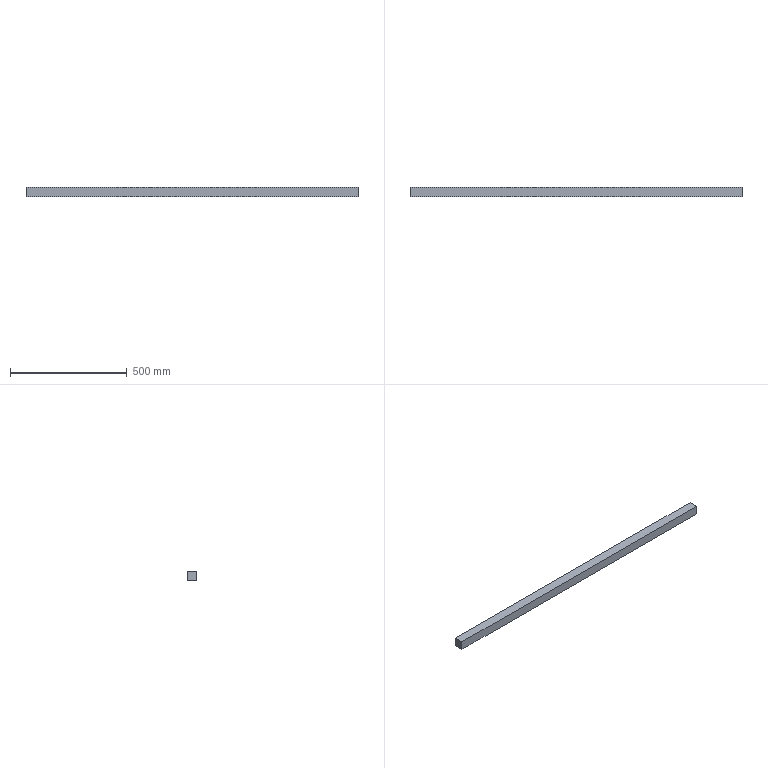Part | NX | features 凸台-拉伸2[1] 2 | 1 solid | 6 faces | box 1420 x 40 x 40 mm | volume 2272000 mm3 | plane 6
STEP:
#1=CARTESIAN_POINT('',(4293.,-600.,1387.015));
#2=VERTEX_POINT('',#1);
#3=CARTESIAN_POINT('',(4293.,-600.,1427.015));
#4=VERTEX_POINT('',#3);
#5=CARTESIAN_POINT('',(4293.,-600.,1427.015));
#6=DIRECTION('',(0.,0.,1.));
#7=VECTOR('',#6,1000.);
#8=LINE('',#5,#7);
#9=EDGE_CURVE('',#2,#4,#8,.T.);
#10=ORIENTED_EDGE('',*,*,#9,.F.);
#11=CARTESIAN_POINT('',(4293.,-560.,1387.015));
#12=VERTEX_POINT('',#11);
#13=CARTESIAN_POINT('',(4293.,-600.,1387.015));
#14=DIRECTION('',(0.,-1.,0.));
#15=VECTOR('',#14,1000.);
#16=LINE('',#13,#15);
#17=EDGE_CURVE('',#12,#2,#16,.T.);
#18=ORIENTED_EDGE('',*,*,#17,.F.);
#19=CARTESIAN_POINT('',(4293.,-560.,1427.015));
#20=VERTEX_POINT('',#19);
#21=CARTESIAN_POINT('',(4293.,-560.,1427.015));
#22=DIRECTION('',(0.,0.,-1.));
#23=VECTOR('',#22,1000.);
#24=LINE('',#21,#23);
#25=EDGE_CURVE('',#20,#12,#24,.T.);
#26=ORIENTED_EDGE('',*,*,#25,.F.);
#27=CARTESIAN_POINT('',(4293.,-600.,1427.015));
#28=DIRECTION('',(0.,1.,0.));
#29=VECTOR('',#28,1000.);
#30=LINE('',#27,#29);
#31=EDGE_CURVE('',#4,#20,#30,.T.);
#32=ORIENTED_EDGE('',*,*,#31,.F.);
#33=EDGE_LOOP('',(#10,#18,#26,#32));
#34=FACE_BOUND('',#33,.T.);
#35=CARTESIAN_POINT('',(4293.,-600.,1427.015));
#36=DIRECTION('',(-1.,0.,0.));
#37=DIRECTION('',(0.,0.,1.));
#38=AXIS2_PLACEMENT_3D('',#35,#36,#37);
#39=PLANE('',#38);
#40=ADVANCED_FACE('',(#34),#39,.F.);
#41=CARTESIAN_POINT('',(2873.,-600.,1427.015));
#42=VERTEX_POINT('',#41);
#43=CARTESIAN_POINT('',(4349.569,-600.,1427.015));
#44=DIRECTION('',(-1.,0.,0.));
#45=VECTOR('',#44,1000.);
#46=LINE('',#43,#45);
#47=EDGE_CURVE('',#4,#42,#46,.T.);
#48=ORIENTED_EDGE('',*,*,#47,.F.);
#49=ORIENTED_EDGE('',*,*,#31,.T.);
#50=CARTESIAN_POINT('',(2873.,-560.,1427.015));
#51=VERTEX_POINT('',#50);
#52=CARTESIAN_POINT('',(4349.569,-560.,1427.015));
#53=DIRECTION('',(-1.,0.,0.));
#54=VECTOR('',#53,1000.);
#55=LINE('',#52,#54);
#56=EDGE_CURVE('',#20,#51,#55,.T.);
#57=ORIENTED_EDGE('',*,*,#56,.T.);
#58=CARTESIAN_POINT('',(2873.,-600.,1427.015));
#59=DIRECTION('',(0.,-1.,0.));
#60=VECTOR('',#59,1000.);
#61=LINE('',#58,#60);
#62=EDGE_CURVE('',#51,#42,#61,.T.);
#63=ORIENTED_EDGE('',*,*,#62,.T.);
#64=EDGE_LOOP('',(#48,#49,#57,#63));
#65=FACE_BOUND('',#64,.T.);
#66=CARTESIAN_POINT('',(4349.569,-600.,1427.015));
#67=DIRECTION('',(0.,0.,-1.));
#68=DIRECTION('',(-1.,0.,0.));
#69=AXIS2_PLACEMENT_3D('',#66,#67,#68);
#70=PLANE('',#69);
#71=ADVANCED_FACE('',(#65),#70,.F.);
#72=CARTESIAN_POINT('',(2873.,-600.,1387.015));
#73=VERTEX_POINT('',#72);
#74=CARTESIAN_POINT('',(4349.569,-600.,1387.015));
#75=DIRECTION('',(-1.,0.,0.));
#76=VECTOR('',#75,1000.);
#77=LINE('',#74,#76);
#78=EDGE_CURVE('',#2,#73,#77,.T.);
#79=ORIENTED_EDGE('',*,*,#78,.F.);
#80=ORIENTED_EDGE('',*,*,#9,.T.);
#81=ORIENTED_EDGE('',*,*,#47,.T.);
#82=CARTESIAN_POINT('',(2873.,-600.,1427.015));
#83=DIRECTION('',(0.,0.,-1.));
#84=VECTOR('',#83,1000.);
#85=LINE('',#82,#84);
#86=EDGE_CURVE('',#42,#73,#85,.T.);
#87=ORIENTED_EDGE('',*,*,#86,.T.);
#88=EDGE_LOOP('',(#79,#80,#81,#87));
#89=FACE_BOUND('',#88,.T.);
#90=CARTESIAN_POINT('',(4349.569,-600.,1427.015));
#91=DIRECTION('',(0.,1.,0.));
#92=DIRECTION('',(0.,0.,1.));
#93=AXIS2_PLACEMENT_3D('',#90,#91,#92);
#94=PLANE('',#93);
#95=ADVANCED_FACE('',(#89),#94,.F.);
#96=CARTESIAN_POINT('',(2873.,-560.,1387.015));
#97=VERTEX_POINT('',#96);
#98=CARTESIAN_POINT('',(4349.569,-560.,1387.015));
#99=DIRECTION('',(-1.,0.,0.));
#100=VECTOR('',#99,1000.);
#101=LINE('',#98,#100);
#102=EDGE_CURVE('',#12,#97,#101,.T.);
#103=ORIENTED_EDGE('',*,*,#102,.F.);
#104=ORIENTED_EDGE('',*,*,#17,.T.);
#105=ORIENTED_EDGE('',*,*,#78,.T.);
#106=CARTESIAN_POINT('',(2873.,-600.,1387.015));
#107=DIRECTION('',(0.,1.,0.));
#108=VECTOR('',#107,1000.);
#109=LINE('',#106,#108);
#110=EDGE_CURVE('',#73,#97,#109,.T.);
#111=ORIENTED_EDGE('',*,*,#110,.T.);
#112=EDGE_LOOP('',(#103,#104,#105,#111));
#113=FACE_BOUND('',#112,.T.);
#114=CARTESIAN_POINT('',(4349.569,-600.,1387.015));
#115=DIRECTION('',(0.,0.,1.));
#116=DIRECTION('',(1.,0.,0.));
#117=AXIS2_PLACEMENT_3D('',#114,#115,#116);
#118=PLANE('',#117);
#119=ADVANCED_FACE('',(#113),#118,.F.);
#120=ORIENTED_EDGE('',*,*,#56,.F.);
#121=ORIENTED_EDGE('',*,*,#25,.T.);
#122=ORIENTED_EDGE('',*,*,#102,.T.);
#123=CARTESIAN_POINT('',(2873.,-560.,1427.015));
#124=DIRECTION('',(0.,0.,1.));
#125=VECTOR('',#124,1000.);
#126=LINE('',#123,#125);
#127=EDGE_CURVE('',#97,#51,#126,.T.);
#128=ORIENTED_EDGE('',*,*,#127,.T.);
#129=EDGE_LOOP('',(#120,#121,#122,#128));
#130=FACE_BOUND('',#129,.T.);
#131=CARTESIAN_POINT('',(4349.569,-560.,1427.015));
#132=DIRECTION('',(0.,-1.,0.));
#133=DIRECTION('',(0.,0.,-1.));
#134=AXIS2_PLACEMENT_3D('',#131,#132,#133);
#135=PLANE('',#134);
#136=ADVANCED_FACE('',(#130),#135,.F.);
#137=ORIENTED_EDGE('',*,*,#62,.F.);
#138=ORIENTED_EDGE('',*,*,#127,.F.);
#139=ORIENTED_EDGE('',*,*,#110,.F.);
#140=ORIENTED_EDGE('',*,*,#86,.F.);
#141=EDGE_LOOP('',(#137,#138,#139,#140));
#142=FACE_BOUND('',#141,.T.);
#143=CARTESIAN_POINT('',(2873.,0.,1400.));
#144=DIRECTION('',(-1.,0.,0.));
#145=DIRECTION('',(0.,0.,1.));
#146=AXIS2_PLACEMENT_3D('',#143,#144,#145);
#147=PLANE('',#146);
#148=ADVANCED_FACE('',(#142),#147,.T.);
#149=CLOSED_SHELL('',(#40,#71,#95,#119,#136,#148));
#150=MANIFOLD_SOLID_BREP('',#149);
#151=(LENGTH_UNIT()NAMED_UNIT(*)SI_UNIT(.MILLI.,.METRE.));
#152=UNCERTAINTY_MEASURE_WITH_UNIT(LENGTH_MEASURE(0.00001),#151,'','');
#153=(NAMED_UNIT(*)PLANE_ANGLE_UNIT()SI_UNIT($,.RADIAN.));
#154=(NAMED_UNIT(*)SI_UNIT($,.STERADIAN.)SOLID_ANGLE_UNIT());
#155=(GEOMETRIC_REPRESENTATION_CONTEXT(3)GLOBAL_UNCERTAINTY_ASSIGNED_CONTEXT((#152))GLOBAL_UNIT_ASSIGNED_CONTEXT((#151,#153,#154))REPRESENTATION_CONTEXT('',''));
#156=ADVANCED_BREP_SHAPE_REPRESENTATION('',(#150),#155);